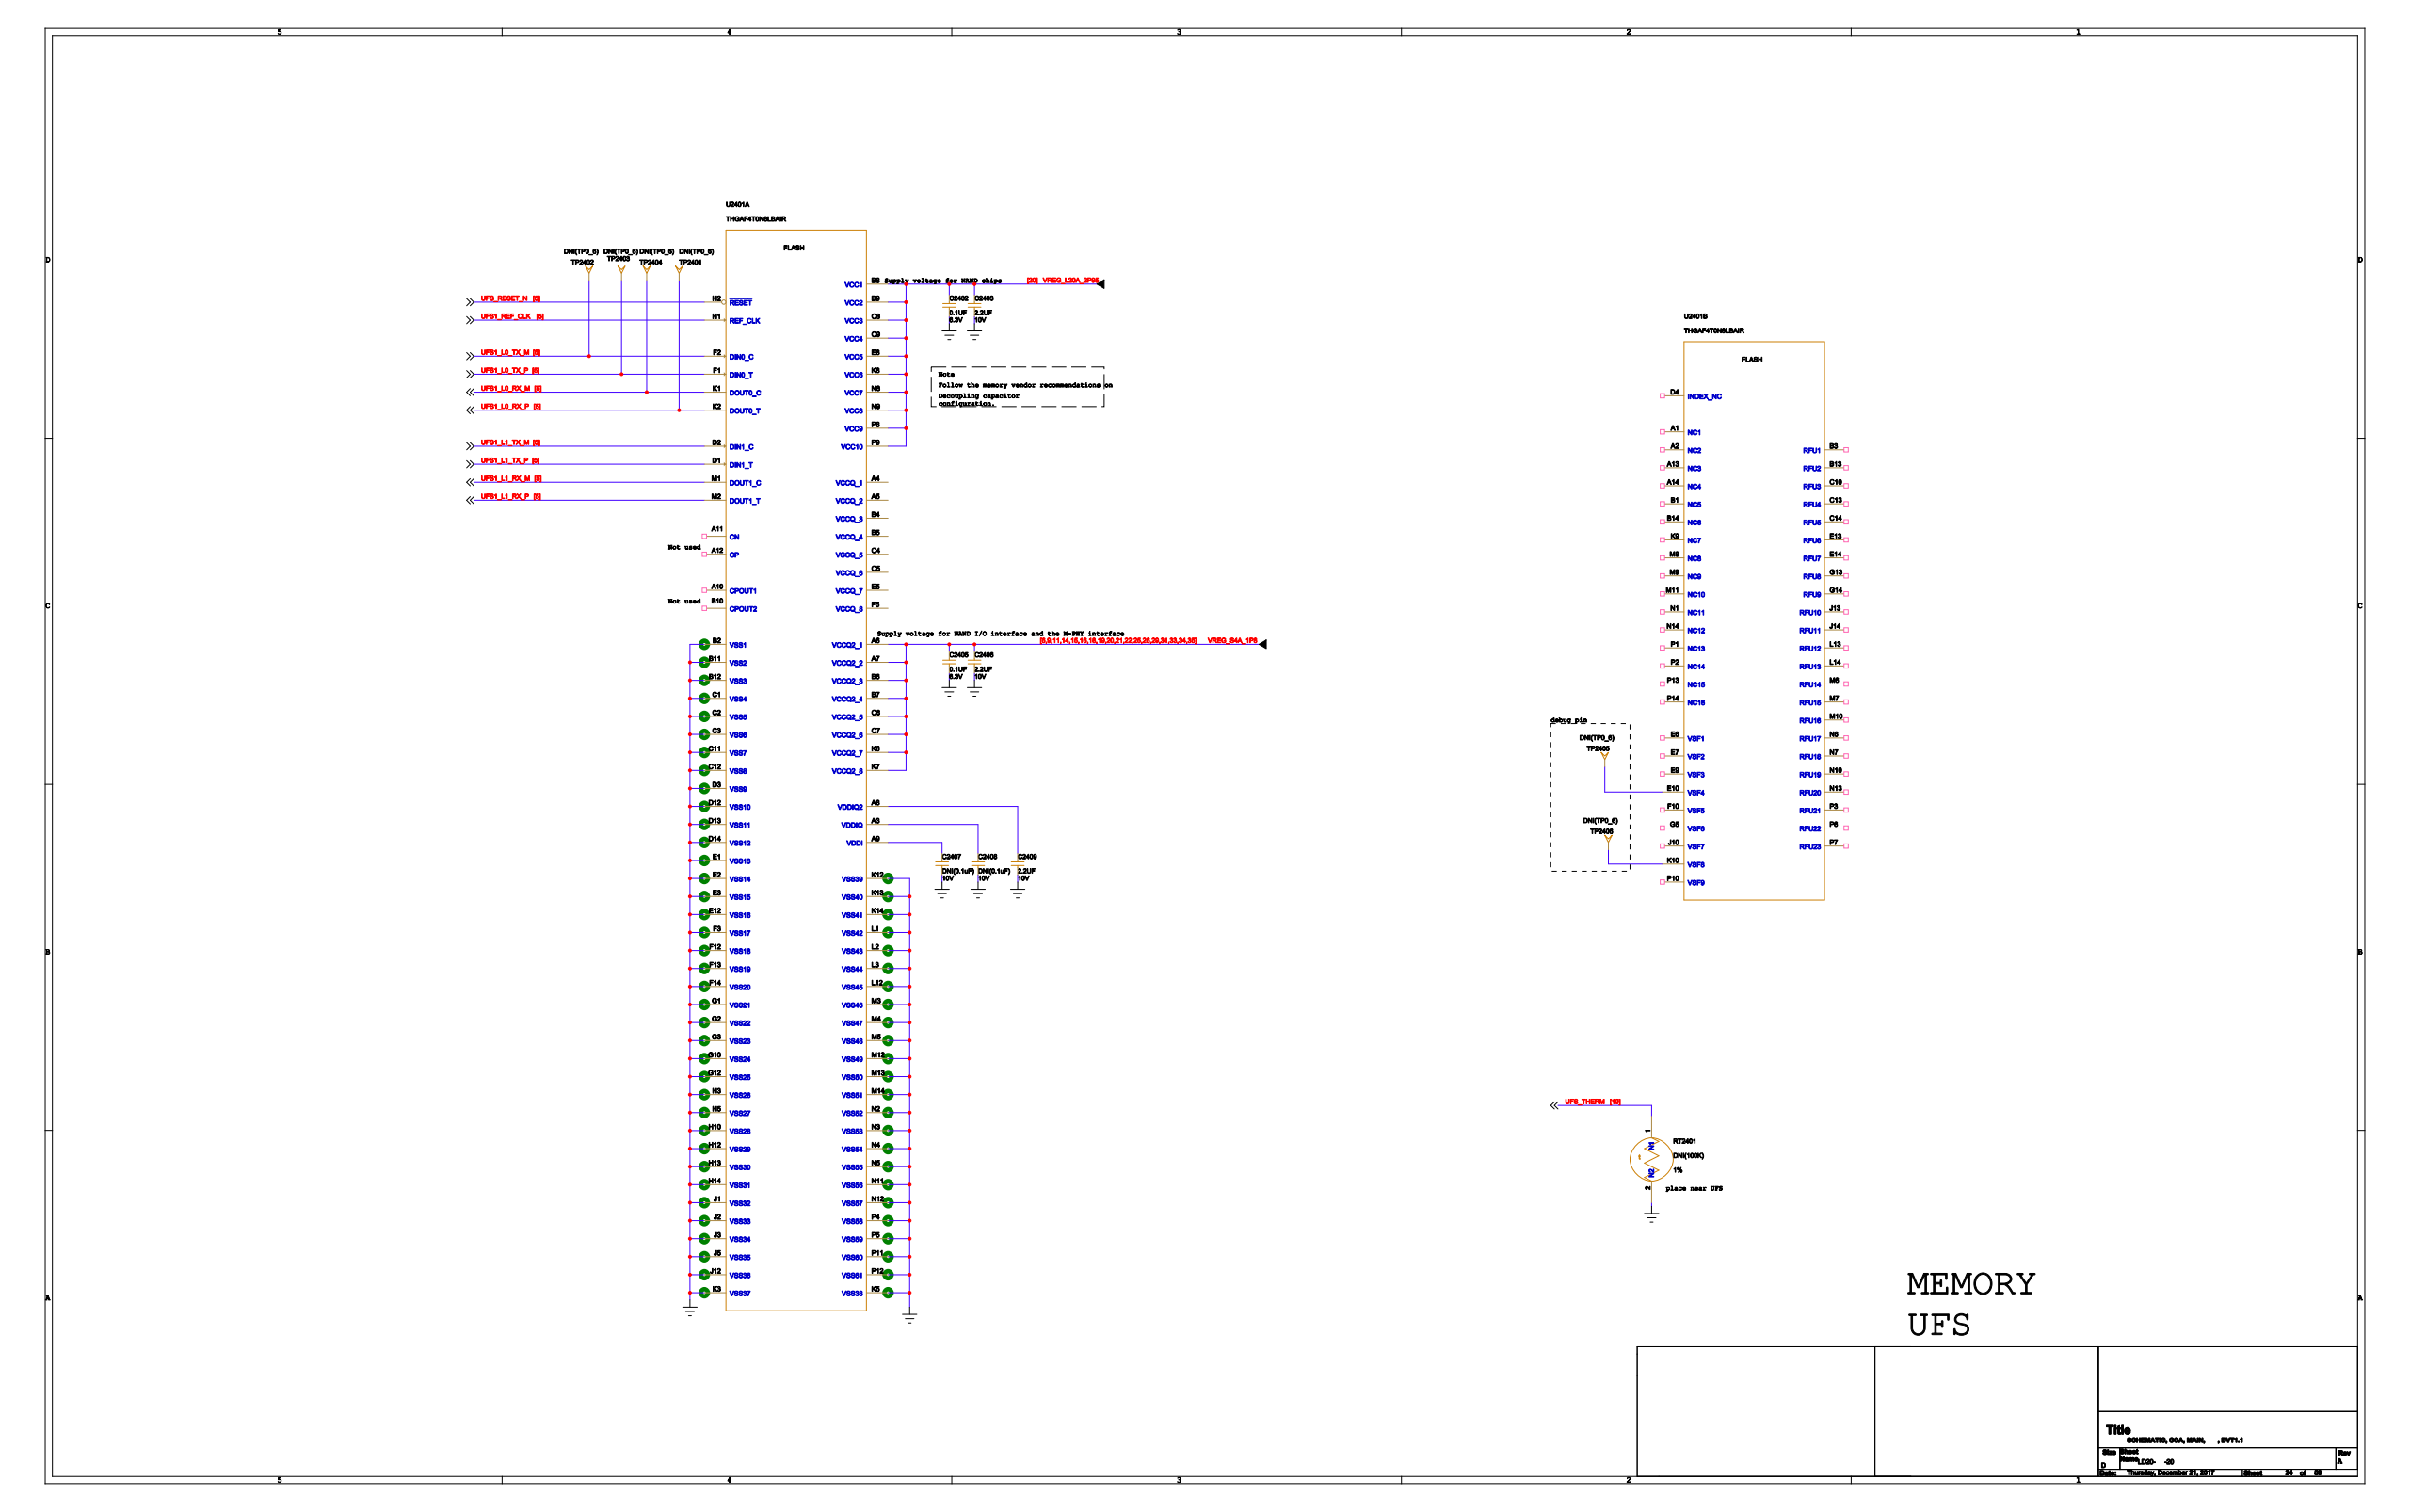Circuit board | Cadence Allegro | 1520 parts | 1149 nets | one sheet of the schematic
Parts on this sheet (reference | value | footprint):
C2402 | 0.1UF | 2P0201R
C2403 | 2.2UF | 2P0402R
C2405 | 0.1UF | 2P0201R
C2406 | 2.2UF | 2P0402R
C2407 | DNI(0.1uF) | 2P0201R_DNI
C2408 | DNI(0.1uF) | 2P0201R_DNI
C2409 | 2.2UF | 2P0402R
RT2401 | DNI(100K) | 2P0201R_DNI
TP2401 | DNI(TP0_6) | TP-0_6
TP2402 | DNI(TP0_6) | TP-0_6
TP2403 | DNI(TP0_6) | TP-0_6
TP2404 | DNI(TP0_6) | TP-0_6
TP2405 | DNI(TP0_6) | TP-0_6
TP2406 | DNI(TP0_6) | TP-0_6
U2401 | THGAF4T0N8LBAIR | 153PGA516X457B197
Nets of these parts (net: part-pin ...):
GND: C2402-2 C2403-2 C2405-2 C2406-2 C2407-2 C2408-2 C2409-2 RT2401-2 U2401-B2 U2401-B11 U2401-B12 U2401-C1 U2401-C2 U2401-C3 U2401-C11 U2401-C12 U2401-D3 U2401-D12 U2401-D13 U2401-D14 U2401-E1 U2401-E2 U2401-E3 U2401-E12 U2401-F3 U2401-F12 U2401-F13 U2401-F14 U2401-G1 U2401-G2 U2401-G3 U2401-G10 U2401-G12 U2401-H3 U2401-H5 U2401-H10 U2401-H12 U2401-H13 U2401-H14 U2401-J1 U2401-J2 U2401-J3 U2401-J5 U2401-J12 U2401-K3 U2401-K5 U2401-K12 U2401-K13 U2401-K14 U2401-L1 U2401-L2 U2401-L3 U2401-L12 U2401-M3 U2401-M4 U2401-M5 U2401-M12 U2401-M13 U2401-M14 U2401-N2 U2401-N3 U2401-N4 U2401-N5 U2401-N11 U2401-N12 U2401-P4 U2401-P5 U2401-P11 U2401-P12
VREG_S4A_1P8: C2405-1 C2406-1 U2401-A6 U2401-A7 U2401-B6 U2401-B7 U2401-C6 U2401-C7 U2401-K6 U2401-K7
VREG_L20A_2P95: C2402-1 C2403-1 U2401-B8 U2401-B9 U2401-C8 U2401-C9 U2401-E8 U2401-K8 U2401-N8 U2401-N9 U2401-P8 U2401-P9
N30722243: C2409-1 U2401-A8
N28735547: C2407-1 U2401-A9
N28735548: C2408-1 U2401-A3
UFS_THERM: RT2401-1
UFS1_L0_RX_P: TP2401-1 U2401-K2
UFS1_L0_TX_M: TP2402-1 U2401-F2
UFS1_L0_TX_P: TP2403-1 U2401-F1
UFS1_L0_RX_M: TP2404-1 U2401-K1
N35607031: TP2405-1 U2401-E10
N35607027: TP2406-1 U2401-K10
UFS1_L1_RX_M: U2401-M1
UFS1_L1_RX_P: U2401-M2
UFS1_L1_TX_M: U2401-D2
UFS1_L1_TX_P: U2401-D1
UFS1_REF_CLK: U2401-H1
UFS_RESET_N: U2401-H2
VCCQ_1: U2401-A4
VCCQ_2: U2401-A5
VCCQ_3: U2401-B4
VCCQ_4: U2401-B5
VCCQ_5: U2401-C4
VCCQ_6: U2401-C5
VCCQ_7: U2401-E5
VCCQ_8: U2401-F5